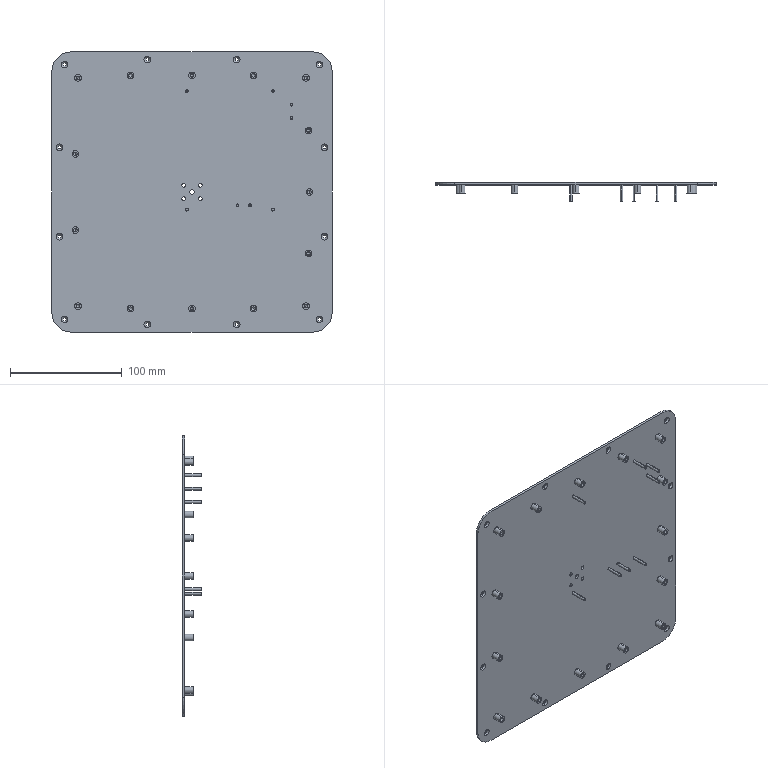Part | SolidWorks | features Chamfer 2, ICE 2, Cut 1, Extrusion 1, HoleWzd 1 | 1 solid | 213 faces | box 250.5 x 17 x 250.5 mm | volume 127405 mm3 | cylinder 114 | cone 70 | plane 29 | commonest cylinder face diameters 3.3 x30 6 x30 3 x24 2.5 x16 3.2 x8 34 x4